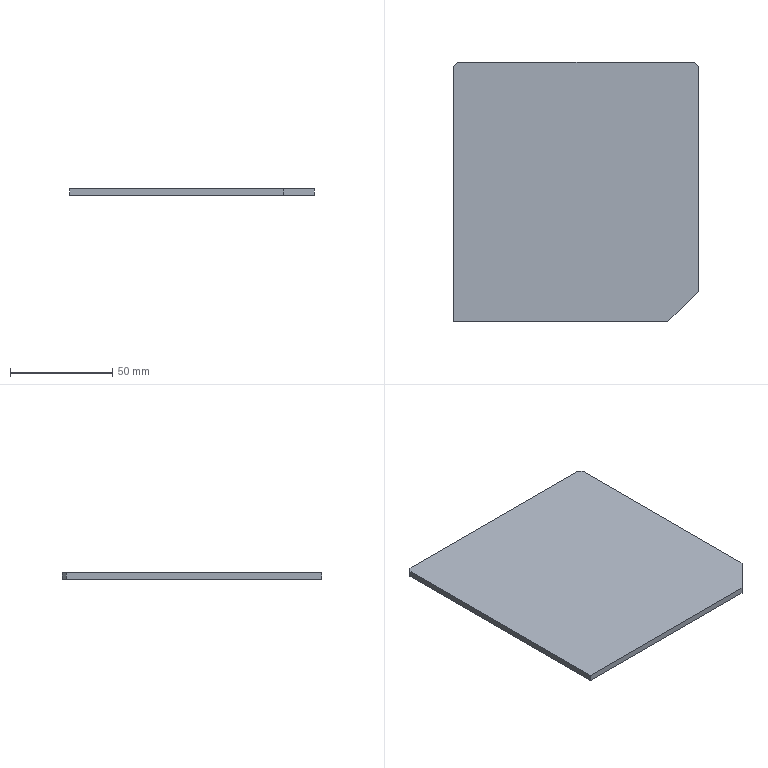Part | SolidWorks | features Chamfer 2, Extrusion 1 | 1 solid | 9 faces | box 120 x 127 x 3 mm | volume 45371 mm3 | plane 9
STEP:
#1=CARTESIAN_POINT('',(-60.,61.5,3.));
#2=VERTEX_POINT('',#1);
#3=CARTESIAN_POINT('',(-60.,-63.5,3.));
#4=VERTEX_POINT('',#3);
#5=CARTESIAN_POINT('',(-60.,63.5,3.));
#6=DIRECTION('',(0.,-1.,0.));
#7=VECTOR('',#6,1000.);
#8=LINE('',#5,#7);
#9=EDGE_CURVE('',#2,#4,#8,.T.);
#10=ORIENTED_EDGE('',*,*,#9,.F.);
#11=CARTESIAN_POINT('',(-60.,61.5,0.));
#12=VERTEX_POINT('',#11);
#13=CARTESIAN_POINT('',(-60.,61.5,3.));
#14=DIRECTION('',(0.,0.,-1.));
#15=VECTOR('',#14,1000.);
#16=LINE('',#13,#15);
#17=EDGE_CURVE('',#2,#12,#16,.T.);
#18=ORIENTED_EDGE('',*,*,#17,.T.);
#19=CARTESIAN_POINT('',(-60.,-63.5,0.));
#20=VERTEX_POINT('',#19);
#21=CARTESIAN_POINT('',(-60.,63.5,0.));
#22=DIRECTION('',(0.,-1.,0.));
#23=VECTOR('',#22,1000.);
#24=LINE('',#21,#23);
#25=EDGE_CURVE('',#12,#20,#24,.T.);
#26=ORIENTED_EDGE('',*,*,#25,.T.);
#27=CARTESIAN_POINT('',(-60.,-63.5,3.));
#28=DIRECTION('',(0.,0.,-1.));
#29=VECTOR('',#28,1000.);
#30=LINE('',#27,#29);
#31=EDGE_CURVE('',#4,#20,#30,.T.);
#32=ORIENTED_EDGE('',*,*,#31,.F.);
#33=EDGE_LOOP('',(#10,#18,#26,#32));
#34=FACE_OUTER_BOUND('',#33,.T.);
#35=CARTESIAN_POINT('',(-60.,63.5,3.));
#36=DIRECTION('',(1.,0.,0.));
#37=DIRECTION('',(0.,1.,0.));
#38=AXIS2_PLACEMENT_3D('',#35,#36,#37);
#39=PLANE('',#38);
#40=ADVANCED_FACE('',(#34),#39,.F.);
#41=CARTESIAN_POINT('',(45.,-63.5,0.));
#42=VERTEX_POINT('',#41);
#43=CARTESIAN_POINT('',(60.,-63.5,0.));
#44=DIRECTION('',(1.,0.,0.));
#45=VECTOR('',#44,1000.);
#46=LINE('',#43,#45);
#47=EDGE_CURVE('',#20,#42,#46,.T.);
#48=ORIENTED_EDGE('',*,*,#47,.T.);
#49=CARTESIAN_POINT('',(45.,-63.5,3.));
#50=VERTEX_POINT('',#49);
#51=CARTESIAN_POINT('',(45.,-63.5,3.));
#52=DIRECTION('',(0.,0.,1.));
#53=VECTOR('',#52,1000.);
#54=LINE('',#51,#53);
#55=EDGE_CURVE('',#42,#50,#54,.T.);
#56=ORIENTED_EDGE('',*,*,#55,.T.);
#57=CARTESIAN_POINT('',(60.,-63.5,3.));
#58=DIRECTION('',(1.,0.,0.));
#59=VECTOR('',#58,1000.);
#60=LINE('',#57,#59);
#61=EDGE_CURVE('',#4,#50,#60,.T.);
#62=ORIENTED_EDGE('',*,*,#61,.F.);
#63=ORIENTED_EDGE('',*,*,#31,.T.);
#64=EDGE_LOOP('',(#48,#56,#62,#63));
#65=FACE_OUTER_BOUND('',#64,.T.);
#66=CARTESIAN_POINT('',(60.,-63.5,3.));
#67=DIRECTION('',(0.,1.,0.));
#68=DIRECTION('',(-1.,0.,0.));
#69=AXIS2_PLACEMENT_3D('',#66,#67,#68);
#70=PLANE('',#69);
#71=ADVANCED_FACE('',(#65),#70,.F.);
#72=CARTESIAN_POINT('',(60.,-48.5,0.));
#73=VERTEX_POINT('',#72);
#74=CARTESIAN_POINT('',(60.,61.5,0.));
#75=VERTEX_POINT('',#74);
#76=CARTESIAN_POINT('',(60.,63.5,0.));
#77=DIRECTION('',(0.,1.,0.));
#78=VECTOR('',#77,1000.);
#79=LINE('',#76,#78);
#80=EDGE_CURVE('',#73,#75,#79,.T.);
#81=ORIENTED_EDGE('',*,*,#80,.T.);
#82=CARTESIAN_POINT('',(60.,61.5,3.));
#83=VERTEX_POINT('',#82);
#84=CARTESIAN_POINT('',(60.,61.5,3.));
#85=DIRECTION('',(0.,0.,1.));
#86=VECTOR('',#85,1000.);
#87=LINE('',#84,#86);
#88=EDGE_CURVE('',#75,#83,#87,.T.);
#89=ORIENTED_EDGE('',*,*,#88,.T.);
#90=CARTESIAN_POINT('',(60.,-48.5,3.));
#91=VERTEX_POINT('',#90);
#92=CARTESIAN_POINT('',(60.,63.5,3.));
#93=DIRECTION('',(0.,1.,0.));
#94=VECTOR('',#93,1000.);
#95=LINE('',#92,#94);
#96=EDGE_CURVE('',#91,#83,#95,.T.);
#97=ORIENTED_EDGE('',*,*,#96,.F.);
#98=CARTESIAN_POINT('',(60.,-48.5,3.));
#99=DIRECTION('',(0.,0.,-1.));
#100=VECTOR('',#99,1000.);
#101=LINE('',#98,#100);
#102=EDGE_CURVE('',#91,#73,#101,.T.);
#103=ORIENTED_EDGE('',*,*,#102,.T.);
#104=EDGE_LOOP('',(#81,#89,#97,#103));
#105=FACE_OUTER_BOUND('',#104,.T.);
#106=CARTESIAN_POINT('',(60.,63.5,3.));
#107=DIRECTION('',(-1.,0.,0.));
#108=DIRECTION('',(0.,-1.,0.));
#109=AXIS2_PLACEMENT_3D('',#106,#107,#108);
#110=PLANE('',#109);
#111=ADVANCED_FACE('',(#105),#110,.F.);
#112=CARTESIAN_POINT('',(58.,63.5,3.));
#113=VERTEX_POINT('',#112);
#114=CARTESIAN_POINT('',(-58.,63.5,3.));
#115=VERTEX_POINT('',#114);
#116=CARTESIAN_POINT('',(60.,63.5,3.));
#117=DIRECTION('',(-1.,0.,0.));
#118=VECTOR('',#117,1000.);
#119=LINE('',#116,#118);
#120=EDGE_CURVE('',#113,#115,#119,.T.);
#121=ORIENTED_EDGE('',*,*,#120,.F.);
#122=CARTESIAN_POINT('',(58.,63.5,0.));
#123=VERTEX_POINT('',#122);
#124=CARTESIAN_POINT('',(58.,63.5,3.));
#125=DIRECTION('',(0.,0.,-1.));
#126=VECTOR('',#125,1000.);
#127=LINE('',#124,#126);
#128=EDGE_CURVE('',#113,#123,#127,.T.);
#129=ORIENTED_EDGE('',*,*,#128,.T.);
#130=CARTESIAN_POINT('',(-58.,63.5,0.));
#131=VERTEX_POINT('',#130);
#132=CARTESIAN_POINT('',(60.,63.5,0.));
#133=DIRECTION('',(-1.,0.,0.));
#134=VECTOR('',#133,1000.);
#135=LINE('',#132,#134);
#136=EDGE_CURVE('',#123,#131,#135,.T.);
#137=ORIENTED_EDGE('',*,*,#136,.T.);
#138=CARTESIAN_POINT('',(-58.,63.5,3.));
#139=DIRECTION('',(0.,0.,1.));
#140=VECTOR('',#139,1000.);
#141=LINE('',#138,#140);
#142=EDGE_CURVE('',#131,#115,#141,.T.);
#143=ORIENTED_EDGE('',*,*,#142,.T.);
#144=EDGE_LOOP('',(#121,#129,#137,#143));
#145=FACE_OUTER_BOUND('',#144,.T.);
#146=CARTESIAN_POINT('',(60.,63.5,3.));
#147=DIRECTION('',(0.,-1.,0.));
#148=DIRECTION('',(1.,0.,0.));
#149=AXIS2_PLACEMENT_3D('',#146,#147,#148);
#150=PLANE('',#149);
#151=ADVANCED_FACE('',(#145),#150,.F.);
#152=ORIENTED_EDGE('',*,*,#96,.T.);
#153=CARTESIAN_POINT('',(58.,63.5,3.));
#154=DIRECTION('',(-0.7071,0.7071,0.));
#155=VECTOR('',#154,1000.);
#156=LINE('',#153,#155);
#157=EDGE_CURVE('',#83,#113,#156,.T.);
#158=ORIENTED_EDGE('',*,*,#157,.T.);
#159=ORIENTED_EDGE('',*,*,#120,.T.);
#160=CARTESIAN_POINT('',(-60.,61.5,3.));
#161=DIRECTION('',(-0.7071,-0.7071,0.));
#162=VECTOR('',#161,1000.);
#163=LINE('',#160,#162);
#164=EDGE_CURVE('',#115,#2,#163,.T.);
#165=ORIENTED_EDGE('',*,*,#164,.T.);
#166=ORIENTED_EDGE('',*,*,#9,.T.);
#167=ORIENTED_EDGE('',*,*,#61,.T.);
#168=CARTESIAN_POINT('',(60.,-48.5,3.));
#169=DIRECTION('',(0.7071,0.7071,0.));
#170=VECTOR('',#169,1000.);
#171=LINE('',#168,#170);
#172=EDGE_CURVE('',#50,#91,#171,.T.);
#173=ORIENTED_EDGE('',*,*,#172,.T.);
#174=EDGE_LOOP('',(#152,#158,#159,#165,#166,#167,#173));
#175=FACE_OUTER_BOUND('',#174,.T.);
#176=CARTESIAN_POINT('',(0.,0.,3.));
#177=DIRECTION('',(0.,0.,-1.));
#178=DIRECTION('',(-1.,0.,0.));
#179=AXIS2_PLACEMENT_3D('',#176,#177,#178);
#180=PLANE('',#179);
#181=ADVANCED_FACE('',(#175),#180,.F.);
#182=ORIENTED_EDGE('',*,*,#136,.F.);
#183=CARTESIAN_POINT('',(60.75,60.75,0.));
#184=DIRECTION('',(0.7071,-0.7071,0.));
#185=VECTOR('',#184,1000.);
#186=LINE('',#183,#185);
#187=EDGE_CURVE('',#123,#75,#186,.T.);
#188=ORIENTED_EDGE('',*,*,#187,.T.);
#189=ORIENTED_EDGE('',*,*,#80,.F.);
#190=CARTESIAN_POINT('',(54.25,-54.25,0.));
#191=DIRECTION('',(-0.7071,-0.7071,0.));
#192=VECTOR('',#191,1000.);
#193=LINE('',#190,#192);
#194=EDGE_CURVE('',#73,#42,#193,.T.);
#195=ORIENTED_EDGE('',*,*,#194,.T.);
#196=ORIENTED_EDGE('',*,*,#47,.F.);
#197=ORIENTED_EDGE('',*,*,#25,.F.);
#198=CARTESIAN_POINT('',(-60.75,60.75,0.));
#199=DIRECTION('',(0.7071,0.7071,0.));
#200=VECTOR('',#199,1000.);
#201=LINE('',#198,#200);
#202=EDGE_CURVE('',#12,#131,#201,.T.);
#203=ORIENTED_EDGE('',*,*,#202,.T.);
#204=EDGE_LOOP('',(#182,#188,#189,#195,#196,#197,#203));
#205=FACE_OUTER_BOUND('',#204,.T.);
#206=CARTESIAN_POINT('',(0.,0.,0.));
#207=DIRECTION('',(0.,0.,-1.));
#208=DIRECTION('',(-1.,0.,0.));
#209=AXIS2_PLACEMENT_3D('',#206,#207,#208);
#210=PLANE('',#209);
#211=ADVANCED_FACE('',(#205),#210,.T.);
#212=ORIENTED_EDGE('',*,*,#172,.F.);
#213=ORIENTED_EDGE('',*,*,#55,.F.);
#214=ORIENTED_EDGE('',*,*,#194,.F.);
#215=ORIENTED_EDGE('',*,*,#102,.F.);
#216=EDGE_LOOP('',(#212,#213,#214,#215));
#217=FACE_OUTER_BOUND('',#216,.T.);
#218=CARTESIAN_POINT('',(60.,-48.5,3.));
#219=DIRECTION('',(-0.7071,0.7071,0.));
#220=DIRECTION('',(0.,0.,-1.));
#221=AXIS2_PLACEMENT_3D('',#218,#219,#220);
#222=PLANE('',#221);
#223=ADVANCED_FACE('',(#217),#222,.F.);
#224=ORIENTED_EDGE('',*,*,#157,.F.);
#225=ORIENTED_EDGE('',*,*,#88,.F.);
#226=ORIENTED_EDGE('',*,*,#187,.F.);
#227=ORIENTED_EDGE('',*,*,#128,.F.);
#228=EDGE_LOOP('',(#224,#225,#226,#227));
#229=FACE_OUTER_BOUND('',#228,.T.);
#230=CARTESIAN_POINT('',(58.,63.5,3.));
#231=DIRECTION('',(-0.7071,-0.7071,0.));
#232=DIRECTION('',(0.,0.,-1.));
#233=AXIS2_PLACEMENT_3D('',#230,#231,#232);
#234=PLANE('',#233);
#235=ADVANCED_FACE('',(#229),#234,.F.);
#236=ORIENTED_EDGE('',*,*,#164,.F.);
#237=ORIENTED_EDGE('',*,*,#142,.F.);
#238=ORIENTED_EDGE('',*,*,#202,.F.);
#239=ORIENTED_EDGE('',*,*,#17,.F.);
#240=EDGE_LOOP('',(#236,#237,#238,#239));
#241=FACE_OUTER_BOUND('',#240,.T.);
#242=CARTESIAN_POINT('',(-60.,61.5,3.));
#243=DIRECTION('',(0.7071,-0.7071,0.));
#244=DIRECTION('',(0.,0.,-1.));
#245=AXIS2_PLACEMENT_3D('',#242,#243,#244);
#246=PLANE('',#245);
#247=ADVANCED_FACE('',(#241),#246,.F.);
#248=CLOSED_SHELL('',(#40,#71,#111,#151,#181,#211,#223,#235,#247));
#249=MANIFOLD_SOLID_BREP('',#248);
#250=CARTESIAN_POINT('',(0.,0.,0.));
#251=DIRECTION('',(0.,0.,1.));
#252=DIRECTION('',(1.,0.,0.));
#253=AXIS2_PLACEMENT_3D('',#250,#251,#252);
#254=(LENGTH_UNIT()NAMED_UNIT(*)SI_UNIT(.MILLI.,.METRE.));
#255=UNCERTAINTY_MEASURE_WITH_UNIT(LENGTH_MEASURE(0.00001),#254,'','');
#256=(NAMED_UNIT(*)PLANE_ANGLE_UNIT()SI_UNIT($,.RADIAN.));
#257=(NAMED_UNIT(*)SI_UNIT($,.STERADIAN.)SOLID_ANGLE_UNIT());
#258=(GEOMETRIC_REPRESENTATION_CONTEXT(3)GLOBAL_UNCERTAINTY_ASSIGNED_CONTEXT((#255))GLOBAL_UNIT_ASSIGNED_CONTEXT((#254,#256,#257))REPRESENTATION_CONTEXT('',''));
#259=ADVANCED_BREP_SHAPE_REPRESENTATION('',(#249,#253),#258);